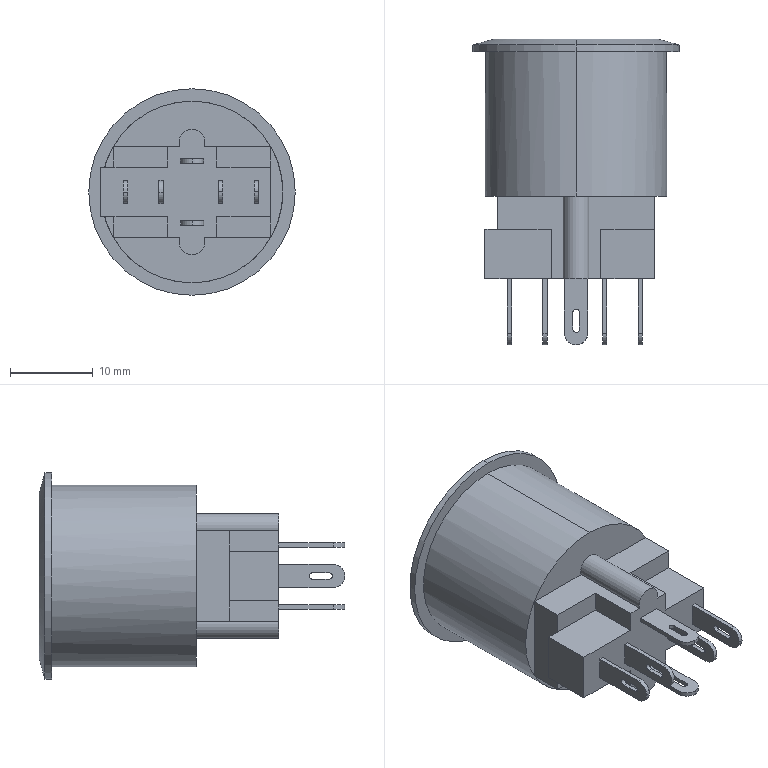Part | SolidWorks | features ICE 10, Fillet 2, LPattern 1, Revolution 1 | 2 solids | 108 faces | box 25 x 37 x 25 mm | volume 9217 mm3 | plane 67 | cylinder 39 | cone 2 | commonest cylinder face diameters 0.8 x12 2.8 x12 18 x4 3.156 x3 13.5 x2 14 x2